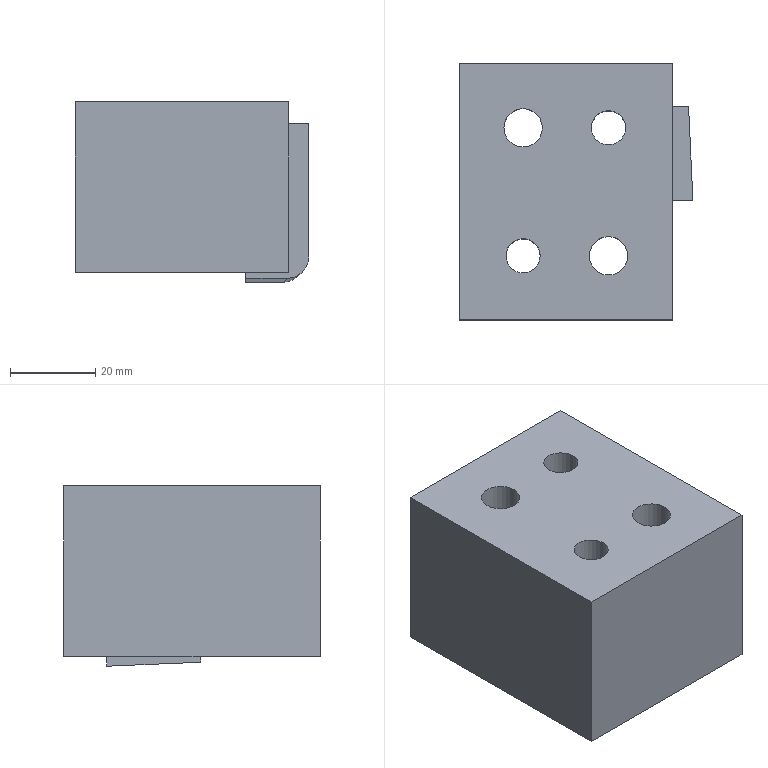Part | NX | features solid 2 | 1 solid | 21 faces | box 54.781 x 60 x 42.28 mm | volume 110990 mm3 | plane 14 | cylinder 7 | commonest cylinder face diameters 8 x2 9 x2 14 x2 10 x1
STEP:
#1=CARTESIAN_POINT('',(1381.,-145.,15.));
#2=VERTEX_POINT('',#1);
#3=CARTESIAN_POINT('',(1385.,-145.,15.));
#4=DIRECTION('',(0.,0.,-1.));
#5=DIRECTION('',(-1.,0.,0.));
#6=AXIS2_PLACEMENT_3D('',#3,#4,#5);
#7=CIRCLE('',#6,4.);
#8=EDGE_CURVE('',#2,#2,#7,.T.);
#9=ORIENTED_EDGE('',*,*,#8,.T.);
#10=EDGE_LOOP('',(#9));
#11=FACE_BOUND('',#10,.T.);
#12=CARTESIAN_POINT('',(1361.,-175.,15.));
#13=VERTEX_POINT('',#12);
#14=CARTESIAN_POINT('',(1365.,-175.,15.));
#15=DIRECTION('',(0.,0.,-1.));
#16=DIRECTION('',(-1.,0.,0.));
#17=AXIS2_PLACEMENT_3D('',#14,#15,#16);
#18=CIRCLE('',#17,4.);
#19=EDGE_CURVE('',#13,#13,#18,.T.);
#20=ORIENTED_EDGE('',*,*,#19,.T.);
#21=EDGE_LOOP('',(#20));
#22=FACE_BOUND('',#21,.T.);
#23=CARTESIAN_POINT('',(1360.5,-145.,15.));
#24=VERTEX_POINT('',#23);
#25=CARTESIAN_POINT('',(1365.,-145.,15.));
#26=DIRECTION('',(0.,0.,-1.));
#27=DIRECTION('',(-1.,0.,0.));
#28=AXIS2_PLACEMENT_3D('',#25,#26,#27);
#29=CIRCLE('',#28,4.5);
#30=EDGE_CURVE('',#24,#24,#29,.T.);
#31=ORIENTED_EDGE('',*,*,#30,.T.);
#32=EDGE_LOOP('',(#31));
#33=FACE_BOUND('',#32,.T.);
#34=CARTESIAN_POINT('',(1380.5,-175.,15.));
#35=VERTEX_POINT('',#34);
#36=CARTESIAN_POINT('',(1385.,-175.,15.));
#37=DIRECTION('',(0.,0.,-1.));
#38=DIRECTION('',(-1.,0.,0.));
#39=AXIS2_PLACEMENT_3D('',#36,#37,#38);
#40=CIRCLE('',#39,4.5);
#41=EDGE_CURVE('',#35,#35,#40,.T.);
#42=ORIENTED_EDGE('',*,*,#41,.T.);
#43=EDGE_LOOP('',(#42));
#44=FACE_BOUND('',#43,.T.);
#45=CARTESIAN_POINT('',(1350.,-190.,15.));
#46=VERTEX_POINT('',#45);
#47=CARTESIAN_POINT('',(1400.,-190.,15.));
#48=VERTEX_POINT('',#47);
#49=CARTESIAN_POINT('',(1360.,-190.,15.));
#50=DIRECTION('',(1.,0.,0.));
#51=VECTOR('',#50,1000.);
#52=LINE('',#49,#51);
#53=EDGE_CURVE('',#46,#48,#52,.T.);
#54=ORIENTED_EDGE('',*,*,#53,.T.);
#55=CARTESIAN_POINT('',(1400.,-130.,15.));
#56=VERTEX_POINT('',#55);
#57=CARTESIAN_POINT('',(1400.,-140.,15.));
#58=DIRECTION('',(0.,-1.,0.));
#59=VECTOR('',#58,1000.);
#60=LINE('',#57,#59);
#61=EDGE_CURVE('',#56,#48,#60,.T.);
#62=ORIENTED_EDGE('',*,*,#61,.F.);
#63=CARTESIAN_POINT('',(1350.,-130.,15.));
#64=VERTEX_POINT('',#63);
#65=CARTESIAN_POINT('',(1360.,-130.,15.));
#66=DIRECTION('',(-1.,0.,0.));
#67=VECTOR('',#66,1000.);
#68=LINE('',#65,#67);
#69=EDGE_CURVE('',#64,#56,#68,.F.);
#70=ORIENTED_EDGE('',*,*,#69,.F.);
#71=CARTESIAN_POINT('',(1350.,-140.,15.));
#72=DIRECTION('',(0.,-1.,0.));
#73=VECTOR('',#72,1000.);
#74=LINE('',#71,#73);
#75=EDGE_CURVE('',#64,#46,#74,.T.);
#76=ORIENTED_EDGE('',*,*,#75,.T.);
#77=EDGE_LOOP('',(#54,#62,#70,#76));
#78=FACE_BOUND('',#77,.T.);
#79=CARTESIAN_POINT('',(1360.,-140.,15.));
#80=DIRECTION('',(0.,0.,1.));
#81=DIRECTION('',(0.,-1.,0.));
#82=AXIS2_PLACEMENT_3D('',#79,#80,#81);
#83=PLANE('',#82);
#84=ADVANCED_FACE('',(#11,#22,#33,#44,#78),#83,.T.);
#85=ORIENTED_EDGE('',*,*,#69,.T.);
#86=CARTESIAN_POINT('',(1400.,-130.,-25.));
#87=VERTEX_POINT('',#86);
#88=CARTESIAN_POINT('',(1400.,-130.,60.));
#89=DIRECTION('',(0.,0.,1.));
#90=VECTOR('',#89,1000.);
#91=LINE('',#88,#90);
#92=EDGE_CURVE('',#56,#87,#91,.F.);
#93=ORIENTED_EDGE('',*,*,#92,.T.);
#94=CARTESIAN_POINT('',(1350.,-130.,-25.));
#95=VERTEX_POINT('',#94);
#96=CARTESIAN_POINT('',(1360.,-130.,-25.));
#97=DIRECTION('',(1.,0.,0.));
#98=VECTOR('',#97,1000.);
#99=LINE('',#96,#98);
#100=EDGE_CURVE('',#95,#87,#99,.T.);
#101=ORIENTED_EDGE('',*,*,#100,.F.);
#102=CARTESIAN_POINT('',(1350.,-130.,60.));
#103=DIRECTION('',(0.,0.,1.));
#104=VECTOR('',#103,1000.);
#105=LINE('',#102,#104);
#106=EDGE_CURVE('',#64,#95,#105,.F.);
#107=ORIENTED_EDGE('',*,*,#106,.F.);
#108=EDGE_LOOP('',(#85,#93,#101,#107));
#109=FACE_BOUND('',#108,.T.);
#110=CARTESIAN_POINT('',(1360.,-130.,60.));
#111=DIRECTION('',(0.,-1.,0.));
#112=DIRECTION('',(0.,0.,-1.));
#113=AXIS2_PLACEMENT_3D('',#110,#111,#112);
#114=PLANE('',#113);
#115=ADVANCED_FACE('',(#109),#114,.F.);
#116=CARTESIAN_POINT('',(1381.,-145.,-25.));
#117=VERTEX_POINT('',#116);
#118=CARTESIAN_POINT('',(1385.,-145.,-25.));
#119=DIRECTION('',(0.,0.,-1.));
#120=DIRECTION('',(-1.,0.,0.));
#121=AXIS2_PLACEMENT_3D('',#118,#119,#120);
#122=CIRCLE('',#121,4.);
#123=EDGE_CURVE('',#117,#117,#122,.T.);
#124=ORIENTED_EDGE('',*,*,#123,.F.);
#125=EDGE_LOOP('',(#124));
#126=FACE_BOUND('',#125,.T.);
#127=CARTESIAN_POINT('',(1361.,-175.,-25.));
#128=VERTEX_POINT('',#127);
#129=CARTESIAN_POINT('',(1365.,-175.,-25.));
#130=DIRECTION('',(0.,0.,-1.));
#131=DIRECTION('',(-1.,0.,0.));
#132=AXIS2_PLACEMENT_3D('',#129,#130,#131);
#133=CIRCLE('',#132,4.);
#134=EDGE_CURVE('',#128,#128,#133,.T.);
#135=ORIENTED_EDGE('',*,*,#134,.F.);
#136=EDGE_LOOP('',(#135));
#137=FACE_BOUND('',#136,.T.);
#138=CARTESIAN_POINT('',(1358.,-145.,-25.));
#139=VERTEX_POINT('',#138);
#140=CARTESIAN_POINT('',(1365.,-145.,-25.));
#141=DIRECTION('',(0.,0.,-1.));
#142=DIRECTION('',(-1.,0.,0.));
#143=AXIS2_PLACEMENT_3D('',#140,#141,#142);
#144=CIRCLE('',#143,7.);
#145=EDGE_CURVE('',#139,#139,#144,.T.);
#146=ORIENTED_EDGE('',*,*,#145,.F.);
#147=EDGE_LOOP('',(#146));
#148=FACE_BOUND('',#147,.T.);
#149=CARTESIAN_POINT('',(1378.,-175.,-25.));
#150=VERTEX_POINT('',#149);
#151=CARTESIAN_POINT('',(1385.,-175.,-25.));
#152=DIRECTION('',(0.,0.,-1.));
#153=DIRECTION('',(-1.,0.,0.));
#154=AXIS2_PLACEMENT_3D('',#151,#152,#153);
#155=CIRCLE('',#154,7.);
#156=EDGE_CURVE('',#150,#150,#155,.T.);
#157=ORIENTED_EDGE('',*,*,#156,.F.);
#158=EDGE_LOOP('',(#157));
#159=FACE_BOUND('',#158,.T.);
#160=CARTESIAN_POINT('',(1400.,-140.,-25.));
#161=VERTEX_POINT('',#160);
#162=CARTESIAN_POINT('',(1390.,-140.,-25.));
#163=VERTEX_POINT('',#162);
#164=CARTESIAN_POINT('',(1360.,-140.,-25.));
#165=DIRECTION('',(1.,0.,0.));
#166=VECTOR('',#165,1000.);
#167=LINE('',#164,#166);
#168=EDGE_CURVE('',#161,#163,#167,.F.);
#169=ORIENTED_EDGE('',*,*,#168,.T.);
#170=CARTESIAN_POINT('',(1390.,-162.,-25.));
#171=VERTEX_POINT('',#170);
#172=CARTESIAN_POINT('',(1390.,-140.,-25.));
#173=DIRECTION('',(0.,-1.,0.));
#174=VECTOR('',#173,1000.);
#175=LINE('',#172,#174);
#176=EDGE_CURVE('',#163,#171,#175,.T.);
#177=ORIENTED_EDGE('',*,*,#176,.T.);
#178=CARTESIAN_POINT('',(1400.,-162.,-25.));
#179=VERTEX_POINT('',#178);
#180=CARTESIAN_POINT('',(1360.,-162.,-25.));
#181=DIRECTION('',(1.,0.,0.));
#182=VECTOR('',#181,1000.);
#183=LINE('',#180,#182);
#184=EDGE_CURVE('',#171,#179,#183,.T.);
#185=ORIENTED_EDGE('',*,*,#184,.T.);
#186=CARTESIAN_POINT('',(1400.,-190.,-25.));
#187=VERTEX_POINT('',#186);
#188=CARTESIAN_POINT('',(1400.,-140.,-25.));
#189=DIRECTION('',(0.,1.,0.));
#190=VECTOR('',#189,1000.);
#191=LINE('',#188,#190);
#192=EDGE_CURVE('',#179,#187,#191,.F.);
#193=ORIENTED_EDGE('',*,*,#192,.T.);
#194=CARTESIAN_POINT('',(1350.,-190.,-25.));
#195=VERTEX_POINT('',#194);
#196=CARTESIAN_POINT('',(1360.,-190.,-25.));
#197=DIRECTION('',(-1.,0.,0.));
#198=VECTOR('',#197,1000.);
#199=LINE('',#196,#198);
#200=EDGE_CURVE('',#195,#187,#199,.F.);
#201=ORIENTED_EDGE('',*,*,#200,.F.);
#202=CARTESIAN_POINT('',(1350.,-140.,-25.));
#203=DIRECTION('',(0.,1.,0.));
#204=VECTOR('',#203,1000.);
#205=LINE('',#202,#204);
#206=EDGE_CURVE('',#95,#195,#205,.F.);
#207=ORIENTED_EDGE('',*,*,#206,.F.);
#208=ORIENTED_EDGE('',*,*,#100,.T.);
#209=CARTESIAN_POINT('',(1400.,-140.,-25.));
#210=DIRECTION('',(0.,1.,0.));
#211=VECTOR('',#210,1000.);
#212=LINE('',#209,#211);
#213=EDGE_CURVE('',#87,#161,#212,.F.);
#214=ORIENTED_EDGE('',*,*,#213,.T.);
#215=EDGE_LOOP('',(#169,#177,#185,#193,#201,#207,#208,#214));
#216=FACE_BOUND('',#215,.T.);
#217=CARTESIAN_POINT('',(1360.,-140.,-25.));
#218=DIRECTION('',(0.,0.,1.));
#219=DIRECTION('',(0.,-1.,0.));
#220=AXIS2_PLACEMENT_3D('',#217,#218,#219);
#221=PLANE('',#220);
#222=ADVANCED_FACE('',(#126,#137,#148,#159,#216),#221,.F.);
#223=CARTESIAN_POINT('',(1350.,-190.,60.));
#224=DIRECTION('',(0.,0.,-1.));
#225=VECTOR('',#224,1000.);
#226=LINE('',#223,#225);
#227=EDGE_CURVE('',#46,#195,#226,.T.);
#228=ORIENTED_EDGE('',*,*,#227,.T.);
#229=ORIENTED_EDGE('',*,*,#200,.T.);
#230=CARTESIAN_POINT('',(1400.,-190.,60.));
#231=DIRECTION('',(0.,0.,-1.));
#232=VECTOR('',#231,1000.);
#233=LINE('',#230,#232);
#234=EDGE_CURVE('',#48,#187,#233,.T.);
#235=ORIENTED_EDGE('',*,*,#234,.F.);
#236=ORIENTED_EDGE('',*,*,#53,.F.);
#237=EDGE_LOOP('',(#228,#229,#235,#236));
#238=FACE_BOUND('',#237,.T.);
#239=CARTESIAN_POINT('',(1360.,-190.,60.));
#240=DIRECTION('',(0.,-1.,0.));
#241=DIRECTION('',(0.,0.,-1.));
#242=AXIS2_PLACEMENT_3D('',#239,#240,#241);
#243=PLANE('',#242);
#244=ADVANCED_FACE('',(#238),#243,.T.);
#245=ORIENTED_EDGE('',*,*,#213,.F.);
#246=ORIENTED_EDGE('',*,*,#92,.F.);
#247=ORIENTED_EDGE('',*,*,#61,.T.);
#248=ORIENTED_EDGE('',*,*,#234,.T.);
#249=ORIENTED_EDGE('',*,*,#192,.F.);
#250=CARTESIAN_POINT('',(1400.,-162.,10.));
#251=VERTEX_POINT('',#250);
#252=CARTESIAN_POINT('',(1400.,-162.,60.));
#253=DIRECTION('',(0.,0.,1.));
#254=VECTOR('',#253,1000.);
#255=LINE('',#252,#254);
#256=EDGE_CURVE('',#251,#179,#255,.F.);
#257=ORIENTED_EDGE('',*,*,#256,.F.);
#258=CARTESIAN_POINT('',(1400.,-140.,10.));
#259=VERTEX_POINT('',#258);
#260=CARTESIAN_POINT('',(1400.,-140.,10.));
#261=DIRECTION('',(0.,-1.,0.));
#262=VECTOR('',#261,1000.);
#263=LINE('',#260,#262);
#264=EDGE_CURVE('',#259,#251,#263,.T.);
#265=ORIENTED_EDGE('',*,*,#264,.F.);
#266=CARTESIAN_POINT('',(1400.,-140.,60.));
#267=DIRECTION('',(0.,0.,1.));
#268=VECTOR('',#267,1000.);
#269=LINE('',#266,#268);
#270=EDGE_CURVE('',#161,#259,#269,.T.);
#271=ORIENTED_EDGE('',*,*,#270,.F.);
#272=EDGE_LOOP('',(#245,#246,#247,#248,#249,#257,#265,#271));
#273=FACE_BOUND('',#272,.T.);
#274=CARTESIAN_POINT('',(1400.,-140.,60.));
#275=DIRECTION('',(-1.,0.,0.));
#276=DIRECTION('',(0.,0.,-1.));
#277=AXIS2_PLACEMENT_3D('',#274,#275,#276);
#278=PLANE('',#277);
#279=ADVANCED_FACE('',(#273),#278,.F.);
#280=ORIENTED_EDGE('',*,*,#206,.T.);
#281=ORIENTED_EDGE('',*,*,#227,.F.);
#282=ORIENTED_EDGE('',*,*,#75,.F.);
#283=ORIENTED_EDGE('',*,*,#106,.T.);
#284=EDGE_LOOP('',(#280,#281,#282,#283));
#285=FACE_BOUND('',#284,.T.);
#286=CARTESIAN_POINT('',(1350.,-140.,60.));
#287=DIRECTION('',(-1.,0.,0.));
#288=DIRECTION('',(0.,0.,-1.));
#289=AXIS2_PLACEMENT_3D('',#286,#287,#288);
#290=PLANE('',#289);
#291=ADVANCED_FACE('',(#285),#290,.T.);
#292=ORIENTED_EDGE('',*,*,#264,.T.);
#293=CARTESIAN_POINT('',(1404.781,-162.,10.));
#294=VERTEX_POINT('',#293);
#295=CARTESIAN_POINT('',(1380.,-162.,10.));
#296=DIRECTION('',(1.,0.,0.));
#297=VECTOR('',#296,1000.);
#298=LINE('',#295,#297);
#299=EDGE_CURVE('',#294,#251,#298,.F.);
#300=ORIENTED_EDGE('',*,*,#299,.F.);
#301=CARTESIAN_POINT('',(1403.762,-140.,10.));
#302=VERTEX_POINT('',#301);
#303=CARTESIAN_POINT('',(1404.623,-158.576,10.));
#304=DIRECTION('',(0.0463,-0.9989,0.));
#305=VECTOR('',#304,1000.);
#306=LINE('',#303,#305);
#307=EDGE_CURVE('',#302,#294,#306,.T.);
#308=ORIENTED_EDGE('',*,*,#307,.F.);
#309=CARTESIAN_POINT('',(1403.097,-140.,10.));
#310=DIRECTION('',(-1.,0.,0.));
#311=VECTOR('',#310,1000.);
#312=LINE('',#309,#311);
#313=EDGE_CURVE('',#302,#259,#312,.T.);
#314=ORIENTED_EDGE('',*,*,#313,.T.);
#315=EDGE_LOOP('',(#292,#300,#308,#314));
#316=FACE_BOUND('',#315,.T.);
#317=CARTESIAN_POINT('',(1380.,-119.951,10.));
#318=DIRECTION('',(0.,0.,1.));
#319=DIRECTION('',(0.,1.,0.));
#320=AXIS2_PLACEMENT_3D('',#317,#318,#319);
#321=PLANE('',#320);
#322=ADVANCED_FACE('',(#316),#321,.T.);
#323=CARTESIAN_POINT('',(1398.696,-140.,-27.277));
#324=VERTEX_POINT('',#323);
#325=CARTESIAN_POINT('',(1390.,-140.,-27.28));
#326=VERTEX_POINT('',#325);
#327=CARTESIAN_POINT('',(1404.445,-140.,-27.275));
#328=DIRECTION('',(-1.,0.,-0.0003531));
#329=VECTOR('',#328,1000.);
#330=LINE('',#327,#329);
#331=EDGE_CURVE('',#324,#326,#330,.T.);
#332=ORIENTED_EDGE('',*,*,#331,.T.);
#333=CARTESIAN_POINT('',(1390.,-140.,-47.208));
#334=DIRECTION('',(0.,0.,-1.));
#335=VECTOR('',#334,1000.);
#336=LINE('',#333,#335);
#337=EDGE_CURVE('',#326,#163,#336,.F.);
#338=ORIENTED_EDGE('',*,*,#337,.T.);
#339=ORIENTED_EDGE('',*,*,#168,.F.);
#340=ORIENTED_EDGE('',*,*,#270,.T.);
#341=ORIENTED_EDGE('',*,*,#313,.F.);
#342=CARTESIAN_POINT('',(1403.709,-140.,-22.271));
#343=VERTEX_POINT('',#342);
#344=CARTESIAN_POINT('',(1403.719,-140.,-16.62));
#345=DIRECTION('',(0.001618,0.,1.));
#346=VECTOR('',#345,1000.);
#347=LINE('',#344,#346);
#348=EDGE_CURVE('',#343,#302,#347,.T.);
#349=ORIENTED_EDGE('',*,*,#348,.F.);
#350=CARTESIAN_POINT('',(1398.704,-140.,-22.273));
#351=DIRECTION('',(0.,-1.,0.));
#352=DIRECTION('',(0.7371,0.,0.6758));
#353=AXIS2_PLACEMENT_3D('',#350,#351,#352);
#354=ELLIPSE('',#353,5.01,5.);
#355=EDGE_CURVE('',#324,#343,#354,.T.);
#356=ORIENTED_EDGE('',*,*,#355,.F.);
#357=EDGE_LOOP('',(#332,#338,#339,#340,#341,#349,#356));
#358=FACE_BOUND('',#357,.T.);
#359=CARTESIAN_POINT('',(1403.097,-140.,172.468));
#360=DIRECTION('',(0.,1.,0.));
#361=DIRECTION('',(1.,0.,0.));
#362=AXIS2_PLACEMENT_3D('',#359,#360,#361);
#363=PLANE('',#362);
#364=ADVANCED_FACE('',(#358),#363,.T.);
#365=CARTESIAN_POINT('',(1404.731,-162.,-21.335));
#366=VERTEX_POINT('',#365);
#367=CARTESIAN_POINT('',(1404.738,-162.,-16.622));
#368=DIRECTION('',(0.001618,0.,1.));
#369=VECTOR('',#368,1000.);
#370=LINE('',#367,#369);
#371=EDGE_CURVE('',#294,#366,#370,.F.);
#372=ORIENTED_EDGE('',*,*,#371,.F.);
#373=ORIENTED_EDGE('',*,*,#299,.T.);
#374=ORIENTED_EDGE('',*,*,#256,.T.);
#375=ORIENTED_EDGE('',*,*,#184,.F.);
#376=CARTESIAN_POINT('',(1390.,-162.,-26.344));
#377=VERTEX_POINT('',#376);
#378=CARTESIAN_POINT('',(1390.,-162.,-47.208));
#379=DIRECTION('',(0.,0.,-1.));
#380=VECTOR('',#379,1000.);
#381=LINE('',#378,#380);
#382=EDGE_CURVE('',#171,#377,#381,.T.);
#383=ORIENTED_EDGE('',*,*,#382,.T.);
#384=CARTESIAN_POINT('',(1399.717,-162.,-26.341));
#385=VERTEX_POINT('',#384);
#386=CARTESIAN_POINT('',(1404.327,-162.,-26.339));
#387=DIRECTION('',(1.,0.,0.0003531));
#388=VECTOR('',#387,1000.);
#389=LINE('',#386,#388);
#390=EDGE_CURVE('',#385,#377,#389,.F.);
#391=ORIENTED_EDGE('',*,*,#390,.F.);
#392=CARTESIAN_POINT('',(1399.725,-162.,-21.336));
#393=DIRECTION('',(0.,-1.,0.));
#394=DIRECTION('',(0.7371,0.,0.6758));
#395=AXIS2_PLACEMENT_3D('',#392,#393,#394);
#396=ELLIPSE('',#395,5.01,5.);
#397=EDGE_CURVE('',#366,#385,#396,.F.);
#398=ORIENTED_EDGE('',*,*,#397,.F.);
#399=EDGE_LOOP('',(#372,#373,#374,#375,#383,#391,#398));
#400=FACE_BOUND('',#399,.T.);
#401=CARTESIAN_POINT('',(1404.256,-162.,173.955));
#402=DIRECTION('',(0.,1.,0.));
#403=DIRECTION('',(1.,0.,0.));
#404=AXIS2_PLACEMENT_3D('',#401,#402,#403);
#405=PLANE('',#404);
#406=ADVANCED_FACE('',(#400),#405,.F.);
#407=ORIENTED_EDGE('',*,*,#390,.T.);
#408=CARTESIAN_POINT('',(1390.,-286.167,-21.062));
#409=DIRECTION('',(0.,-0.9991,0.0425));
#410=VECTOR('',#409,1000.);
#411=LINE('',#408,#410);
#412=EDGE_CURVE('',#377,#326,#411,.F.);
#413=ORIENTED_EDGE('',*,*,#412,.T.);
#414=ORIENTED_EDGE('',*,*,#331,.F.);
#415=CARTESIAN_POINT('',(1398.707,-140.231,-27.267));
#416=DIRECTION('',(-0.04632,0.998,-0.04247));
#417=VECTOR('',#416,1000.);
#418=LINE('',#415,#417);
#419=EDGE_CURVE('',#385,#324,#418,.T.);
#420=ORIENTED_EDGE('',*,*,#419,.F.);
#421=EDGE_LOOP('',(#407,#413,#414,#420));
#422=FACE_BOUND('',#421,.T.);
#423=CARTESIAN_POINT('',(1404.445,-156.027,-26.593));
#424=DIRECTION('',(0.0003527,-0.0425,-0.9991));
#425=DIRECTION('',(0.,0.9991,-0.0425));
#426=AXIS2_PLACEMENT_3D('',#423,#424,#425);
#427=PLANE('',#426);
#428=ADVANCED_FACE('',(#422),#427,.T.);
#429=ORIENTED_EDGE('',*,*,#348,.T.);
#430=ORIENTED_EDGE('',*,*,#307,.T.);
#431=ORIENTED_EDGE('',*,*,#371,.T.);
#432=CARTESIAN_POINT('',(1404.721,-161.788,-21.344));
#433=DIRECTION('',(-0.04632,0.998,-0.04247));
#434=VECTOR('',#433,1000.);
#435=LINE('',#432,#434);
#436=EDGE_CURVE('',#343,#366,#435,.F.);
#437=ORIENTED_EDGE('',*,*,#436,.F.);
#438=EDGE_LOOP('',(#429,#430,#431,#437));
#439=FACE_BOUND('',#438,.T.);
#440=CARTESIAN_POINT('',(1404.58,-158.578,-16.622));
#441=DIRECTION('',(-0.9989,-0.0463,0.001617));
#442=DIRECTION('',(-0.04633,0.9983,-0.03486));
#443=AXIS2_PLACEMENT_3D('',#440,#441,#442);
#444=PLANE('',#443);
#445=ADVANCED_FACE('',(#439),#444,.F.);
#446=ORIENTED_EDGE('',*,*,#337,.F.);
#447=ORIENTED_EDGE('',*,*,#412,.F.);
#448=ORIENTED_EDGE('',*,*,#382,.F.);
#449=ORIENTED_EDGE('',*,*,#176,.F.);
#450=EDGE_LOOP('',(#446,#447,#448,#449));
#451=FACE_BOUND('',#450,.T.);
#452=CARTESIAN_POINT('',(1390.,-287.279,-47.208));
#453=DIRECTION('',(1.,0.,0.));
#454=DIRECTION('',(0.,-1.,0.));
#455=AXIS2_PLACEMENT_3D('',#452,#453,#454);
#456=PLANE('',#455);
#457=ADVANCED_FACE('',(#451),#456,.F.);
#458=ORIENTED_EDGE('',*,*,#397,.T.);
#459=ORIENTED_EDGE('',*,*,#419,.T.);
#460=ORIENTED_EDGE('',*,*,#355,.T.);
#461=ORIENTED_EDGE('',*,*,#436,.T.);
#462=EDGE_LOOP('',(#458,#459,#460,#461));
#463=FACE_BOUND('',#462,.T.);
#464=CARTESIAN_POINT('',(1399.449,-156.046,-21.59));
#465=DIRECTION('',(0.04632,-0.998,0.04247));
#466=DIRECTION('',(-0.9989,-0.04637,0.));
#467=AXIS2_PLACEMENT_3D('',#464,#465,#466);
#468=CYLINDRICAL_SURFACE('',#467,5.);
#469=ADVANCED_FACE('',(#463),#468,.T.);
#470=ORIENTED_EDGE('',*,*,#41,.F.);
#471=EDGE_LOOP('',(#470));
#472=FACE_BOUND('',#471,.T.);
#473=CARTESIAN_POINT('',(1380.5,-175.,-5.));
#474=VERTEX_POINT('',#473);
#475=CARTESIAN_POINT('',(1385.,-175.,-5.));
#476=DIRECTION('',(0.,0.,-1.));
#477=DIRECTION('',(-1.,0.,0.));
#478=AXIS2_PLACEMENT_3D('',#475,#476,#477);
#479=CIRCLE('',#478,4.5);
#480=EDGE_CURVE('',#474,#474,#479,.T.);
#481=ORIENTED_EDGE('',*,*,#480,.T.);
#482=EDGE_LOOP('',(#481));
#483=FACE_BOUND('',#482,.T.);
#484=CARTESIAN_POINT('',(1385.,-175.,25.));
#485=DIRECTION('',(0.,0.,1.));
#486=DIRECTION('',(-1.,0.,0.));
#487=AXIS2_PLACEMENT_3D('',#484,#485,#486);
#488=CYLINDRICAL_SURFACE('',#487,4.5);
#489=ADVANCED_FACE('',(#472,#483),#488,.F.);
#490=ORIENTED_EDGE('',*,*,#480,.F.);
#491=EDGE_LOOP('',(#490));
#492=FACE_BOUND('',#491,.T.);
#493=CARTESIAN_POINT('',(1378.,-175.,-5.));
#494=VERTEX_POINT('',#493);
#495=CARTESIAN_POINT('',(1385.,-175.,-5.));
#496=DIRECTION('',(0.,0.,-1.));
#497=DIRECTION('',(-1.,0.,0.));
#498=AXIS2_PLACEMENT_3D('',#495,#496,#497);
#499=CIRCLE('',#498,7.);
#500=EDGE_CURVE('',#494,#494,#499,.T.);
#501=ORIENTED_EDGE('',*,*,#500,.T.);
#502=EDGE_LOOP('',(#501));
#503=FACE_BOUND('',#502,.T.);
#504=CARTESIAN_POINT('',(1385.,-175.,-5.));
#505=DIRECTION('',(0.,0.,1.));
#506=DIRECTION('',(-1.,0.,0.));
#507=AXIS2_PLACEMENT_3D('',#504,#505,#506);
#508=PLANE('',#507);
#509=ADVANCED_FACE('',(#492,#503),#508,.F.);
#510=ORIENTED_EDGE('',*,*,#500,.F.);
#511=EDGE_LOOP('',(#510));
#512=FACE_BOUND('',#511,.T.);
#513=ORIENTED_EDGE('',*,*,#156,.T.);
#514=EDGE_LOOP('',(#513));
#515=FACE_BOUND('',#514,.T.);
#516=CARTESIAN_POINT('',(1385.,-175.,-25.));
#517=DIRECTION('',(0.,0.,1.));
#518=DIRECTION('',(-1.,0.,0.));
#519=AXIS2_PLACEMENT_3D('',#516,#517,#518);
#520=CYLINDRICAL_SURFACE('',#519,7.);
#521=ADVANCED_FACE('',(#512,#515),#520,.F.);
#522=ORIENTED_EDGE('',*,*,#30,.F.);
#523=EDGE_LOOP('',(#522));
#524=FACE_BOUND('',#523,.T.);
#525=CARTESIAN_POINT('',(1360.5,-145.,-5.));
#526=VERTEX_POINT('',#525);
#527=CARTESIAN_POINT('',(1365.,-145.,-5.));
#528=DIRECTION('',(0.,0.,-1.));
#529=DIRECTION('',(-1.,0.,0.));
#530=AXIS2_PLACEMENT_3D('',#527,#528,#529);
#531=CIRCLE('',#530,4.5);
#532=EDGE_CURVE('',#526,#526,#531,.T.);
#533=ORIENTED_EDGE('',*,*,#532,.T.);
#534=EDGE_LOOP('',(#533));
#535=FACE_BOUND('',#534,.T.);
#536=CARTESIAN_POINT('',(1365.,-145.,25.));
#537=DIRECTION('',(0.,0.,1.));
#538=DIRECTION('',(-1.,0.,0.));
#539=AXIS2_PLACEMENT_3D('',#536,#537,#538);
#540=CYLINDRICAL_SURFACE('',#539,4.5);
#541=ADVANCED_FACE('',(#524,#535),#540,.F.);
#542=ORIENTED_EDGE('',*,*,#532,.F.);
#543=EDGE_LOOP('',(#542));
#544=FACE_BOUND('',#543,.T.);
#545=CARTESIAN_POINT('',(1358.,-145.,-5.));
#546=VERTEX_POINT('',#545);
#547=CARTESIAN_POINT('',(1365.,-145.,-5.));
#548=DIRECTION('',(0.,0.,-1.));
#549=DIRECTION('',(-1.,0.,0.));
#550=AXIS2_PLACEMENT_3D('',#547,#548,#549);
#551=CIRCLE('',#550,7.);
#552=EDGE_CURVE('',#546,#546,#551,.T.);
#553=ORIENTED_EDGE('',*,*,#552,.T.);
#554=EDGE_LOOP('',(#553));
#555=FACE_BOUND('',#554,.T.);
#556=CARTESIAN_POINT('',(1365.,-145.,-5.));
#557=DIRECTION('',(0.,0.,1.));
#558=DIRECTION('',(-1.,0.,0.));
#559=AXIS2_PLACEMENT_3D('',#556,#557,#558);
#560=PLANE('',#559);
#561=ADVANCED_FACE('',(#544,#555),#560,.F.);
#562=ORIENTED_EDGE('',*,*,#552,.F.);
#563=EDGE_LOOP('',(#562));
#564=FACE_BOUND('',#563,.T.);
#565=ORIENTED_EDGE('',*,*,#145,.T.);
#566=EDGE_LOOP('',(#565));
#567=FACE_BOUND('',#566,.T.);
#568=CARTESIAN_POINT('',(1365.,-145.,-25.));
#569=DIRECTION('',(0.,0.,1.));
#570=DIRECTION('',(-1.,0.,0.));
#571=AXIS2_PLACEMENT_3D('',#568,#569,#570);
#572=CYLINDRICAL_SURFACE('',#571,7.);
#573=ADVANCED_FACE('',(#564,#567),#572,.F.);
#574=ORIENTED_EDGE('',*,*,#19,.F.);
#575=EDGE_LOOP('',(#574));
#576=FACE_BOUND('',#575,.T.);
#577=ORIENTED_EDGE('',*,*,#134,.T.);
#578=EDGE_LOOP('',(#577));
#579=FACE_BOUND('',#578,.T.);
#580=CARTESIAN_POINT('',(1365.,-175.,-25.));
#581=DIRECTION('',(0.,0.,1.));
#582=DIRECTION('',(-1.,0.,0.));
#583=AXIS2_PLACEMENT_3D('',#580,#581,#582);
#584=CYLINDRICAL_SURFACE('',#583,4.);
#585=ADVANCED_FACE('',(#576,#579),#584,.F.);
#586=ORIENTED_EDGE('',*,*,#8,.F.);
#587=EDGE_LOOP('',(#586));
#588=FACE_BOUND('',#587,.T.);
#589=ORIENTED_EDGE('',*,*,#123,.T.);
#590=EDGE_LOOP('',(#589));
#591=FACE_BOUND('',#590,.T.);
#592=CARTESIAN_POINT('',(1385.,-145.,-25.));
#593=DIRECTION('',(0.,0.,1.));
#594=DIRECTION('',(-1.,0.,0.));
#595=AXIS2_PLACEMENT_3D('',#592,#593,#594);
#596=CYLINDRICAL_SURFACE('',#595,4.);
#597=ADVANCED_FACE('',(#588,#591),#596,.F.);
#598=CLOSED_SHELL('',(#84,#115,#222,#244,#279,#291,#322,#364,#406,#428,#445,#457,#469,#489,#509,#521,#541,#561,#573,#585,#597));
#599=MANIFOLD_SOLID_BREP('',#598);
#600=(LENGTH_UNIT()NAMED_UNIT(*)SI_UNIT(.MILLI.,.METRE.));
#601=UNCERTAINTY_MEASURE_WITH_UNIT(LENGTH_MEASURE(0.00001),#600,'','');
#602=(NAMED_UNIT(*)PLANE_ANGLE_UNIT()SI_UNIT($,.RADIAN.));
#603=(NAMED_UNIT(*)SI_UNIT($,.STERADIAN.)SOLID_ANGLE_UNIT());
#604=(GEOMETRIC_REPRESENTATION_CONTEXT(3)GLOBAL_UNCERTAINTY_ASSIGNED_CONTEXT((#601))GLOBAL_UNIT_ASSIGNED_CONTEXT((#600,#602,#603))REPRESENTATION_CONTEXT('',''));
#605=ADVANCED_BREP_SHAPE_REPRESENTATION('',(#599),#604);